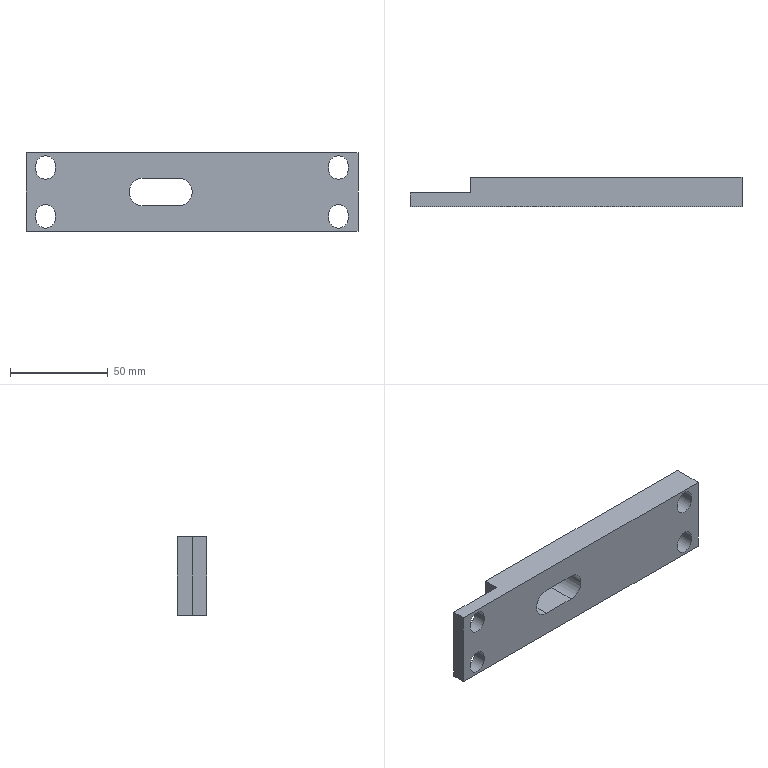Part | SolidWorks | features BaseBody 1 | 1 solid | 32 faces | box 170 x 15 x 40 mm | volume 81474 mm3 | plane 18 | cylinder 14 | commonest cylinder face diameters 10 x12 14.3 x2
STEP:
#1=CARTESIAN_POINT('',(-75.,0.,-6.5));
#2=VERTEX_POINT('',#1);
#3=CARTESIAN_POINT('',(-70.,0.,-11.5));
#4=VERTEX_POINT('',#3);
#5=CARTESIAN_POINT('',(-75.,0.,-11.5));
#6=DIRECTION('',(0.,1.,0.));
#7=DIRECTION('',(0.,0.,1.));
#8=AXIS2_PLACEMENT_3D('',#5,#6,#7);
#9=CIRCLE('',#8,5.);
#10=EDGE_CURVE('',#2,#4,#9,.T.);
#11=ORIENTED_EDGE('',*,*,#10,.F.);
#12=CARTESIAN_POINT('',(-75.,7.,-6.5));
#13=VERTEX_POINT('',#12);
#14=CARTESIAN_POINT('',(-75.,0.,-6.5));
#15=DIRECTION('',(0.,1.,0.));
#16=VECTOR('',#15,1000.);
#17=LINE('',#14,#16);
#18=EDGE_CURVE('',#2,#13,#17,.T.);
#19=ORIENTED_EDGE('',*,*,#18,.T.);
#20=CARTESIAN_POINT('',(-70.,7.,-11.5));
#21=VERTEX_POINT('',#20);
#22=CARTESIAN_POINT('',(-75.,7.,-11.5));
#23=DIRECTION('',(0.,-1.,0.));
#24=DIRECTION('',(0.,0.,1.));
#25=AXIS2_PLACEMENT_3D('',#22,#23,#24);
#26=CIRCLE('',#25,5.);
#27=EDGE_CURVE('',#21,#13,#26,.T.);
#28=ORIENTED_EDGE('',*,*,#27,.F.);
#29=CARTESIAN_POINT('',(-70.,0.,-11.5));
#30=DIRECTION('',(0.,-1.,0.));
#31=VECTOR('',#30,1000.);
#32=LINE('',#29,#31);
#33=EDGE_CURVE('',#21,#4,#32,.T.);
#34=ORIENTED_EDGE('',*,*,#33,.T.);
#35=EDGE_LOOP('',(#11,#19,#28,#34));
#36=FACE_OUTER_BOUND('',#35,.T.);
#37=CARTESIAN_POINT('',(-75.,0.,-11.5));
#38=DIRECTION('',(0.,1.,0.));
#39=DIRECTION('',(0.,0.,1.));
#40=AXIS2_PLACEMENT_3D('',#37,#38,#39);
#41=CYLINDRICAL_SURFACE('',#40,5.);
#42=ADVANCED_FACE('',(#36),#41,.F.);
#43=CARTESIAN_POINT('',(75.,0.,18.5));
#44=VERTEX_POINT('',#43);
#45=CARTESIAN_POINT('',(80.,0.,13.5));
#46=VERTEX_POINT('',#45);
#47=CARTESIAN_POINT('',(75.,0.,13.5));
#48=DIRECTION('',(0.,1.,0.));
#49=DIRECTION('',(0.,0.,1.));
#50=AXIS2_PLACEMENT_3D('',#47,#48,#49);
#51=CIRCLE('',#50,5.);
#52=EDGE_CURVE('',#44,#46,#51,.T.);
#53=ORIENTED_EDGE('',*,*,#52,.F.);
#54=CARTESIAN_POINT('',(75.,15.,18.5));
#55=VERTEX_POINT('',#54);
#56=CARTESIAN_POINT('',(75.,0.,18.5));
#57=DIRECTION('',(0.,1.,0.));
#58=VECTOR('',#57,1000.);
#59=LINE('',#56,#58);
#60=EDGE_CURVE('',#44,#55,#59,.T.);
#61=ORIENTED_EDGE('',*,*,#60,.T.);
#62=CARTESIAN_POINT('',(80.,15.,13.5));
#63=VERTEX_POINT('',#62);
#64=CARTESIAN_POINT('',(75.,15.,13.5));
#65=DIRECTION('',(0.,-1.,0.));
#66=DIRECTION('',(0.,0.,1.));
#67=AXIS2_PLACEMENT_3D('',#64,#65,#66);
#68=CIRCLE('',#67,5.);
#69=EDGE_CURVE('',#63,#55,#68,.T.);
#70=ORIENTED_EDGE('',*,*,#69,.F.);
#71=CARTESIAN_POINT('',(80.,0.,13.5));
#72=DIRECTION('',(0.,-1.,0.));
#73=VECTOR('',#72,1000.);
#74=LINE('',#71,#73);
#75=EDGE_CURVE('',#63,#46,#74,.T.);
#76=ORIENTED_EDGE('',*,*,#75,.T.);
#77=EDGE_LOOP('',(#53,#61,#70,#76));
#78=FACE_OUTER_BOUND('',#77,.T.);
#79=CARTESIAN_POINT('',(75.,0.,13.5));
#80=DIRECTION('',(0.,1.,0.));
#81=DIRECTION('',(0.,0.,1.));
#82=AXIS2_PLACEMENT_3D('',#79,#80,#81);
#83=CYLINDRICAL_SURFACE('',#82,5.);
#84=ADVANCED_FACE('',(#78),#83,.F.);
#85=CARTESIAN_POINT('',(-75.,0.,18.5));
#86=VERTEX_POINT('',#85);
#87=CARTESIAN_POINT('',(-70.,0.,13.5));
#88=VERTEX_POINT('',#87);
#89=CARTESIAN_POINT('',(-75.,0.,13.5));
#90=DIRECTION('',(0.,1.,0.));
#91=DIRECTION('',(0.,0.,1.));
#92=AXIS2_PLACEMENT_3D('',#89,#90,#91);
#93=CIRCLE('',#92,5.);
#94=EDGE_CURVE('',#86,#88,#93,.T.);
#95=ORIENTED_EDGE('',*,*,#94,.F.);
#96=CARTESIAN_POINT('',(-75.,7.,18.5));
#97=VERTEX_POINT('',#96);
#98=CARTESIAN_POINT('',(-75.,0.,18.5));
#99=DIRECTION('',(0.,1.,0.));
#100=VECTOR('',#99,1000.);
#101=LINE('',#98,#100);
#102=EDGE_CURVE('',#86,#97,#101,.T.);
#103=ORIENTED_EDGE('',*,*,#102,.T.);
#104=CARTESIAN_POINT('',(-70.,7.,13.5));
#105=VERTEX_POINT('',#104);
#106=CARTESIAN_POINT('',(-75.,7.,13.5));
#107=DIRECTION('',(0.,-1.,0.));
#108=DIRECTION('',(0.,0.,1.));
#109=AXIS2_PLACEMENT_3D('',#106,#107,#108);
#110=CIRCLE('',#109,5.);
#111=EDGE_CURVE('',#105,#97,#110,.T.);
#112=ORIENTED_EDGE('',*,*,#111,.F.);
#113=CARTESIAN_POINT('',(-70.,0.,13.5));
#114=DIRECTION('',(0.,-1.,0.));
#115=VECTOR('',#114,1000.);
#116=LINE('',#113,#115);
#117=EDGE_CURVE('',#105,#88,#116,.T.);
#118=ORIENTED_EDGE('',*,*,#117,.T.);
#119=EDGE_LOOP('',(#95,#103,#112,#118));
#120=FACE_OUTER_BOUND('',#119,.T.);
#121=CARTESIAN_POINT('',(-75.,0.,13.5));
#122=DIRECTION('',(0.,1.,0.));
#123=DIRECTION('',(0.,0.,1.));
#124=AXIS2_PLACEMENT_3D('',#121,#122,#123);
#125=CYLINDRICAL_SURFACE('',#124,5.);
#126=ADVANCED_FACE('',(#120),#125,.F.);
#127=CARTESIAN_POINT('',(75.,0.,-6.5));
#128=VERTEX_POINT('',#127);
#129=CARTESIAN_POINT('',(80.,0.,-11.5));
#130=VERTEX_POINT('',#129);
#131=CARTESIAN_POINT('',(75.,0.,-11.5));
#132=DIRECTION('',(0.,1.,0.));
#133=DIRECTION('',(0.,0.,1.));
#134=AXIS2_PLACEMENT_3D('',#131,#132,#133);
#135=CIRCLE('',#134,5.);
#136=EDGE_CURVE('',#128,#130,#135,.T.);
#137=ORIENTED_EDGE('',*,*,#136,.F.);
#138=CARTESIAN_POINT('',(75.,15.,-6.5));
#139=VERTEX_POINT('',#138);
#140=CARTESIAN_POINT('',(75.,0.,-6.5));
#141=DIRECTION('',(0.,1.,0.));
#142=VECTOR('',#141,1000.);
#143=LINE('',#140,#142);
#144=EDGE_CURVE('',#128,#139,#143,.T.);
#145=ORIENTED_EDGE('',*,*,#144,.T.);
#146=CARTESIAN_POINT('',(80.,15.,-11.5));
#147=VERTEX_POINT('',#146);
#148=CARTESIAN_POINT('',(75.,15.,-11.5));
#149=DIRECTION('',(0.,-1.,0.));
#150=DIRECTION('',(0.,0.,1.));
#151=AXIS2_PLACEMENT_3D('',#148,#149,#150);
#152=CIRCLE('',#151,5.);
#153=EDGE_CURVE('',#147,#139,#152,.T.);
#154=ORIENTED_EDGE('',*,*,#153,.F.);
#155=CARTESIAN_POINT('',(80.,0.,-11.5));
#156=DIRECTION('',(0.,-1.,0.));
#157=VECTOR('',#156,1000.);
#158=LINE('',#155,#157);
#159=EDGE_CURVE('',#147,#130,#158,.T.);
#160=ORIENTED_EDGE('',*,*,#159,.T.);
#161=EDGE_LOOP('',(#137,#145,#154,#160));
#162=FACE_OUTER_BOUND('',#161,.T.);
#163=CARTESIAN_POINT('',(75.,0.,-11.5));
#164=DIRECTION('',(0.,1.,0.));
#165=DIRECTION('',(0.,0.,1.));
#166=AXIS2_PLACEMENT_3D('',#163,#164,#165);
#167=CYLINDRICAL_SURFACE('',#166,5.);
#168=ADVANCED_FACE('',(#162),#167,.F.);
#169=CARTESIAN_POINT('',(-85.,0.,20.));
#170=VERTEX_POINT('',#169);
#171=CARTESIAN_POINT('',(-85.,0.,-20.));
#172=VERTEX_POINT('',#171);
#173=CARTESIAN_POINT('',(-85.,0.,0.));
#174=DIRECTION('',(0.,0.,-1.));
#175=VECTOR('',#174,1000.);
#176=LINE('',#173,#175);
#177=EDGE_CURVE('',#170,#172,#176,.T.);
#178=ORIENTED_EDGE('',*,*,#177,.T.);
#179=CARTESIAN_POINT('',(85.,0.,-20.));
#180=VERTEX_POINT('',#179);
#181=CARTESIAN_POINT('',(0.,0.,-20.));
#182=DIRECTION('',(1.,0.,0.));
#183=VECTOR('',#182,1000.);
#184=LINE('',#181,#183);
#185=EDGE_CURVE('',#172,#180,#184,.T.);
#186=ORIENTED_EDGE('',*,*,#185,.T.);
#187=CARTESIAN_POINT('',(85.,0.,20.));
#188=VERTEX_POINT('',#187);
#189=CARTESIAN_POINT('',(85.,0.,0.));
#190=DIRECTION('',(0.,0.,1.));
#191=VECTOR('',#190,1000.);
#192=LINE('',#189,#191);
#193=EDGE_CURVE('',#180,#188,#192,.T.);
#194=ORIENTED_EDGE('',*,*,#193,.T.);
#195=CARTESIAN_POINT('',(0.,0.,20.));
#196=DIRECTION('',(-1.,0.,0.));
#197=VECTOR('',#196,1000.);
#198=LINE('',#195,#197);
#199=EDGE_CURVE('',#188,#170,#198,.T.);
#200=ORIENTED_EDGE('',*,*,#199,.T.);
#201=EDGE_LOOP('',(#178,#186,#194,#200));
#202=FACE_OUTER_BOUND('',#201,.T.);
#203=CARTESIAN_POINT('',(-25.,0.,-7.15));
#204=VERTEX_POINT('',#203);
#205=CARTESIAN_POINT('',(-25.,0.,7.15));
#206=VERTEX_POINT('',#205);
#207=CARTESIAN_POINT('',(-25.,0.,0.));
#208=DIRECTION('',(0.,1.,0.));
#209=DIRECTION('',(0.,0.,1.));
#210=AXIS2_PLACEMENT_3D('',#207,#208,#209);
#211=CIRCLE('',#210,7.15);
#212=EDGE_CURVE('',#204,#206,#211,.T.);
#213=ORIENTED_EDGE('',*,*,#212,.T.);
#214=CARTESIAN_POINT('',(-7.,0.,7.15));
#215=VERTEX_POINT('',#214);
#216=CARTESIAN_POINT('',(0.,0.,7.15));
#217=DIRECTION('',(1.,0.,0.));
#218=VECTOR('',#217,1000.);
#219=LINE('',#216,#218);
#220=EDGE_CURVE('',#206,#215,#219,.T.);
#221=ORIENTED_EDGE('',*,*,#220,.T.);
#222=CARTESIAN_POINT('',(-7.,0.,-7.15));
#223=VERTEX_POINT('',#222);
#224=CARTESIAN_POINT('',(-7.,0.,0.));
#225=DIRECTION('',(0.,1.,0.));
#226=DIRECTION('',(0.,0.,1.));
#227=AXIS2_PLACEMENT_3D('',#224,#225,#226);
#228=CIRCLE('',#227,7.15);
#229=EDGE_CURVE('',#215,#223,#228,.T.);
#230=ORIENTED_EDGE('',*,*,#229,.T.);
#231=CARTESIAN_POINT('',(0.,0.,-7.15));
#232=DIRECTION('',(-1.,0.,0.));
#233=VECTOR('',#232,1000.);
#234=LINE('',#231,#233);
#235=EDGE_CURVE('',#223,#204,#234,.T.);
#236=ORIENTED_EDGE('',*,*,#235,.T.);
#237=EDGE_LOOP('',(#213,#221,#230,#236));
#238=FACE_BOUND('',#237,.T.);
#239=CARTESIAN_POINT('',(-80.,0.,-11.5));
#240=VERTEX_POINT('',#239);
#241=CARTESIAN_POINT('',(-75.,0.,-11.5));
#242=DIRECTION('',(0.,1.,0.));
#243=DIRECTION('',(0.,0.,1.));
#244=AXIS2_PLACEMENT_3D('',#241,#242,#243);
#245=CIRCLE('',#244,5.);
#246=EDGE_CURVE('',#240,#2,#245,.T.);
#247=ORIENTED_EDGE('',*,*,#246,.T.);
#248=ORIENTED_EDGE('',*,*,#10,.T.);
#249=CARTESIAN_POINT('',(-70.,0.,-13.5));
#250=VERTEX_POINT('',#249);
#251=CARTESIAN_POINT('',(-70.,0.,0.));
#252=DIRECTION('',(0.,0.,-1.));
#253=VECTOR('',#252,1000.);
#254=LINE('',#251,#253);
#255=EDGE_CURVE('',#4,#250,#254,.T.);
#256=ORIENTED_EDGE('',*,*,#255,.T.);
#257=CARTESIAN_POINT('',(-80.,0.,-13.5));
#258=VERTEX_POINT('',#257);
#259=CARTESIAN_POINT('',(-75.,0.,-13.5));
#260=DIRECTION('',(0.,1.,0.));
#261=DIRECTION('',(0.,0.,1.));
#262=AXIS2_PLACEMENT_3D('',#259,#260,#261);
#263=CIRCLE('',#262,5.);
#264=EDGE_CURVE('',#250,#258,#263,.T.);
#265=ORIENTED_EDGE('',*,*,#264,.T.);
#266=CARTESIAN_POINT('',(-80.,0.,0.));
#267=DIRECTION('',(0.,0.,1.));
#268=VECTOR('',#267,1000.);
#269=LINE('',#266,#268);
#270=EDGE_CURVE('',#258,#240,#269,.T.);
#271=ORIENTED_EDGE('',*,*,#270,.T.);
#272=EDGE_LOOP('',(#247,#248,#256,#265,#271));
#273=FACE_BOUND('',#272,.T.);
#274=CARTESIAN_POINT('',(80.,0.,11.5));
#275=VERTEX_POINT('',#274);
#276=CARTESIAN_POINT('',(70.,0.,11.5));
#277=VERTEX_POINT('',#276);
#278=CARTESIAN_POINT('',(75.,0.,11.5));
#279=DIRECTION('',(0.,1.,0.));
#280=DIRECTION('',(0.,0.,1.));
#281=AXIS2_PLACEMENT_3D('',#278,#279,#280);
#282=CIRCLE('',#281,5.);
#283=EDGE_CURVE('',#275,#277,#282,.T.);
#284=ORIENTED_EDGE('',*,*,#283,.T.);
#285=CARTESIAN_POINT('',(70.,0.,13.5));
#286=VERTEX_POINT('',#285);
#287=CARTESIAN_POINT('',(70.,0.,0.));
#288=DIRECTION('',(0.,0.,1.));
#289=VECTOR('',#288,1000.);
#290=LINE('',#287,#289);
#291=EDGE_CURVE('',#277,#286,#290,.T.);
#292=ORIENTED_EDGE('',*,*,#291,.T.);
#293=CARTESIAN_POINT('',(75.,0.,13.5));
#294=DIRECTION('',(0.,1.,0.));
#295=DIRECTION('',(0.,0.,1.));
#296=AXIS2_PLACEMENT_3D('',#293,#294,#295);
#297=CIRCLE('',#296,5.);
#298=EDGE_CURVE('',#286,#44,#297,.T.);
#299=ORIENTED_EDGE('',*,*,#298,.T.);
#300=ORIENTED_EDGE('',*,*,#52,.T.);
#301=CARTESIAN_POINT('',(80.,0.,0.));
#302=DIRECTION('',(0.,0.,-1.));
#303=VECTOR('',#302,1000.);
#304=LINE('',#301,#303);
#305=EDGE_CURVE('',#46,#275,#304,.T.);
#306=ORIENTED_EDGE('',*,*,#305,.T.);
#307=EDGE_LOOP('',(#284,#292,#299,#300,#306));
#308=FACE_BOUND('',#307,.T.);
#309=CARTESIAN_POINT('',(-70.,0.,11.5));
#310=VERTEX_POINT('',#309);
#311=CARTESIAN_POINT('',(-80.,0.,11.5));
#312=VERTEX_POINT('',#311);
#313=CARTESIAN_POINT('',(-75.,0.,11.5));
#314=DIRECTION('',(0.,1.,0.));
#315=DIRECTION('',(0.,0.,1.));
#316=AXIS2_PLACEMENT_3D('',#313,#314,#315);
#317=CIRCLE('',#316,5.);
#318=EDGE_CURVE('',#310,#312,#317,.T.);
#319=ORIENTED_EDGE('',*,*,#318,.T.);
#320=CARTESIAN_POINT('',(-80.,0.,13.5));
#321=VERTEX_POINT('',#320);
#322=CARTESIAN_POINT('',(-80.,0.,0.));
#323=DIRECTION('',(0.,0.,1.));
#324=VECTOR('',#323,1000.);
#325=LINE('',#322,#324);
#326=EDGE_CURVE('',#312,#321,#325,.T.);
#327=ORIENTED_EDGE('',*,*,#326,.T.);
#328=CARTESIAN_POINT('',(-75.,0.,13.5));
#329=DIRECTION('',(0.,1.,0.));
#330=DIRECTION('',(0.,0.,1.));
#331=AXIS2_PLACEMENT_3D('',#328,#329,#330);
#332=CIRCLE('',#331,5.);
#333=EDGE_CURVE('',#321,#86,#332,.T.);
#334=ORIENTED_EDGE('',*,*,#333,.T.);
#335=ORIENTED_EDGE('',*,*,#94,.T.);
#336=CARTESIAN_POINT('',(-70.,0.,0.));
#337=DIRECTION('',(0.,0.,-1.));
#338=VECTOR('',#337,1000.);
#339=LINE('',#336,#338);
#340=EDGE_CURVE('',#88,#310,#339,.T.);
#341=ORIENTED_EDGE('',*,*,#340,.T.);
#342=EDGE_LOOP('',(#319,#327,#334,#335,#341));
#343=FACE_BOUND('',#342,.T.);
#344=CARTESIAN_POINT('',(70.,0.,-11.5));
#345=VERTEX_POINT('',#344);
#346=CARTESIAN_POINT('',(75.,0.,-11.5));
#347=DIRECTION('',(0.,1.,0.));
#348=DIRECTION('',(0.,0.,1.));
#349=AXIS2_PLACEMENT_3D('',#346,#347,#348);
#350=CIRCLE('',#349,5.);
#351=EDGE_CURVE('',#345,#128,#350,.T.);
#352=ORIENTED_EDGE('',*,*,#351,.T.);
#353=ORIENTED_EDGE('',*,*,#136,.T.);
#354=CARTESIAN_POINT('',(80.,0.,-13.5));
#355=VERTEX_POINT('',#354);
#356=CARTESIAN_POINT('',(80.,0.,0.));
#357=DIRECTION('',(0.,0.,-1.));
#358=VECTOR('',#357,1000.);
#359=LINE('',#356,#358);
#360=EDGE_CURVE('',#130,#355,#359,.T.);
#361=ORIENTED_EDGE('',*,*,#360,.T.);
#362=CARTESIAN_POINT('',(70.,0.,-13.5));
#363=VERTEX_POINT('',#362);
#364=CARTESIAN_POINT('',(75.,0.,-13.5));
#365=DIRECTION('',(0.,1.,0.));
#366=DIRECTION('',(0.,0.,1.));
#367=AXIS2_PLACEMENT_3D('',#364,#365,#366);
#368=CIRCLE('',#367,5.);
#369=EDGE_CURVE('',#355,#363,#368,.T.);
#370=ORIENTED_EDGE('',*,*,#369,.T.);
#371=CARTESIAN_POINT('',(70.,0.,0.));
#372=DIRECTION('',(0.,0.,1.));
#373=VECTOR('',#372,1000.);
#374=LINE('',#371,#373);
#375=EDGE_CURVE('',#363,#345,#374,.T.);
#376=ORIENTED_EDGE('',*,*,#375,.T.);
#377=EDGE_LOOP('',(#352,#353,#361,#370,#376));
#378=FACE_BOUND('',#377,.T.);
#379=CARTESIAN_POINT('',(0.,0.,0.));
#380=DIRECTION('',(0.,-1.,0.));
#381=DIRECTION('',(0.,0.,-1.));
#382=AXIS2_PLACEMENT_3D('',#379,#380,#381);
#383=PLANE('',#382);
#384=ADVANCED_FACE('',(#202,#238,#273,#308,#343,#378),#383,.T.);
#385=CARTESIAN_POINT('',(-54.,15.,-20.));
#386=VERTEX_POINT('',#385);
#387=CARTESIAN_POINT('',(-54.,7.,-20.));
#388=VERTEX_POINT('',#387);
#389=CARTESIAN_POINT('',(-54.,15.,-20.));
#390=DIRECTION('',(0.,-1.,0.));
#391=VECTOR('',#390,1000.);
#392=LINE('',#389,#391);
#393=EDGE_CURVE('',#386,#388,#392,.T.);
#394=ORIENTED_EDGE('',*,*,#393,.F.);
#395=CARTESIAN_POINT('',(85.,15.,-20.));
#396=VERTEX_POINT('',#395);
#397=CARTESIAN_POINT('',(-85.,15.,-20.));
#398=DIRECTION('',(-1.,0.,0.));
#399=VECTOR('',#398,1000.);
#400=LINE('',#397,#399);
#401=EDGE_CURVE('',#396,#386,#400,.T.);
#402=ORIENTED_EDGE('',*,*,#401,.F.);
#403=CARTESIAN_POINT('',(85.,15.,-20.));
#404=DIRECTION('',(0.,1.,0.));
#405=VECTOR('',#404,1000.);
#406=LINE('',#403,#405);
#407=EDGE_CURVE('',#180,#396,#406,.T.);
#408=ORIENTED_EDGE('',*,*,#407,.F.);
#409=ORIENTED_EDGE('',*,*,#185,.F.);
#410=CARTESIAN_POINT('',(-85.,7.,-20.));
#411=VERTEX_POINT('',#410);
#412=CARTESIAN_POINT('',(-85.,15.,-20.));
#413=DIRECTION('',(0.,-1.,0.));
#414=VECTOR('',#413,1000.);
#415=LINE('',#412,#414);
#416=EDGE_CURVE('',#411,#172,#415,.T.);
#417=ORIENTED_EDGE('',*,*,#416,.F.);
#418=CARTESIAN_POINT('',(-85.,7.,-20.));
#419=DIRECTION('',(-1.,0.,0.));
#420=VECTOR('',#419,1000.);
#421=LINE('',#418,#420);
#422=EDGE_CURVE('',#388,#411,#421,.T.);
#423=ORIENTED_EDGE('',*,*,#422,.F.);
#424=EDGE_LOOP('',(#394,#402,#408,#409,#417,#423));
#425=FACE_OUTER_BOUND('',#424,.T.);
#426=CARTESIAN_POINT('',(-85.,15.,-20.));
#427=DIRECTION('',(0.,0.,1.));
#428=DIRECTION('',(1.,0.,0.));
#429=AXIS2_PLACEMENT_3D('',#426,#427,#428);
#430=PLANE('',#429);
#431=ADVANCED_FACE('',(#425),#430,.F.);
#432=CARTESIAN_POINT('',(-85.,7.,20.));
#433=VERTEX_POINT('',#432);
#434=CARTESIAN_POINT('',(-85.,7.,20.));
#435=DIRECTION('',(0.,0.,1.));
#436=VECTOR('',#435,1000.);
#437=LINE('',#434,#436);
#438=EDGE_CURVE('',#411,#433,#437,.T.);
#439=ORIENTED_EDGE('',*,*,#438,.F.);
#440=ORIENTED_EDGE('',*,*,#416,.T.);
#441=ORIENTED_EDGE('',*,*,#177,.F.);
#442=CARTESIAN_POINT('',(-85.,15.,20.));
#443=DIRECTION('',(0.,-1.,0.));
#444=VECTOR('',#443,1000.);
#445=LINE('',#442,#444);
#446=EDGE_CURVE('',#433,#170,#445,.T.);
#447=ORIENTED_EDGE('',*,*,#446,.F.);
#448=EDGE_LOOP('',(#439,#440,#441,#447));
#449=FACE_OUTER_BOUND('',#448,.T.);
#450=CARTESIAN_POINT('',(-85.,15.,20.));
#451=DIRECTION('',(1.,0.,0.));
#452=DIRECTION('',(0.,0.,-1.));
#453=AXIS2_PLACEMENT_3D('',#450,#451,#452);
#454=PLANE('',#453);
#455=ADVANCED_FACE('',(#449),#454,.F.);
#456=CARTESIAN_POINT('',(-54.,7.,20.));
#457=VERTEX_POINT('',#456);
#458=CARTESIAN_POINT('',(-54.,15.,20.));
#459=VERTEX_POINT('',#458);
#460=CARTESIAN_POINT('',(-54.,15.,20.));
#461=DIRECTION('',(0.,1.,0.));
#462=VECTOR('',#461,1000.);
#463=LINE('',#460,#462);
#464=EDGE_CURVE('',#457,#459,#463,.T.);
#465=ORIENTED_EDGE('',*,*,#464,.F.);
#466=CARTESIAN_POINT('',(-85.,7.,20.));
#467=DIRECTION('',(1.,0.,0.));
#468=VECTOR('',#467,1000.);
#469=LINE('',#466,#468);
#470=EDGE_CURVE('',#433,#457,#469,.T.);
#471=ORIENTED_EDGE('',*,*,#470,.F.);
#472=ORIENTED_EDGE('',*,*,#446,.T.);
#473=ORIENTED_EDGE('',*,*,#199,.F.);
#474=CARTESIAN_POINT('',(85.,15.,20.));
#475=VERTEX_POINT('',#474);
#476=CARTESIAN_POINT('',(85.,15.,20.));
#477=DIRECTION('',(0.,-1.,0.));
#478=VECTOR('',#477,1000.);
#479=LINE('',#476,#478);
#480=EDGE_CURVE('',#475,#188,#479,.T.);
#481=ORIENTED_EDGE('',*,*,#480,.F.);
#482=CARTESIAN_POINT('',(-85.,15.,20.));
#483=DIRECTION('',(1.,0.,0.));
#484=VECTOR('',#483,1000.);
#485=LINE('',#482,#484);
#486=EDGE_CURVE('',#459,#475,#485,.T.);
#487=ORIENTED_EDGE('',*,*,#486,.F.);
#488=EDGE_LOOP('',(#465,#471,#472,#473,#481,#487));
#489=FACE_OUTER_BOUND('',#488,.T.);
#490=CARTESIAN_POINT('',(-85.,15.,20.));
#491=DIRECTION('',(0.,0.,-1.));
#492=DIRECTION('',(-1.,0.,0.));
#493=AXIS2_PLACEMENT_3D('',#490,#491,#492);
#494=PLANE('',#493);
#495=ADVANCED_FACE('',(#489),#494,.F.);
#496=ORIENTED_EDGE('',*,*,#407,.T.);
#497=CARTESIAN_POINT('',(85.,15.,20.));
#498=DIRECTION('',(0.,0.,-1.));
#499=VECTOR('',#498,1000.);
#500=LINE('',#497,#499);
#501=EDGE_CURVE('',#475,#396,#500,.T.);
#502=ORIENTED_EDGE('',*,*,#501,.F.);
#503=ORIENTED_EDGE('',*,*,#480,.T.);
#504=ORIENTED_EDGE('',*,*,#193,.F.);
#505=EDGE_LOOP('',(#496,#502,#503,#504));
#506=FACE_OUTER_BOUND('',#505,.T.);
#507=CARTESIAN_POINT('',(85.,15.,20.));
#508=DIRECTION('',(-1.,0.,0.));
#509=DIRECTION('',(0.,0.,1.));
#510=AXIS2_PLACEMENT_3D('',#507,#508,#509);
#511=PLANE('',#510);
#512=ADVANCED_FACE('',(#506),#511,.F.);
#513=CARTESIAN_POINT('',(-7.,15.,7.15));
#514=VERTEX_POINT('',#513);
#515=CARTESIAN_POINT('',(-7.,0.,7.15));
#516=DIRECTION('',(0.,1.,0.));
#517=VECTOR('',#516,1000.);
#518=LINE('',#515,#517);
#519=EDGE_CURVE('',#215,#514,#518,.T.);
#520=ORIENTED_EDGE('',*,*,#519,.F.);
#521=ORIENTED_EDGE('',*,*,#220,.F.);
#522=CARTESIAN_POINT('',(-25.,15.,7.15));
#523=VERTEX_POINT('',#522);
#524=CARTESIAN_POINT('',(-25.,0.,7.15));
#525=DIRECTION('',(0.,-1.,0.));
#526=VECTOR('',#525,1000.);
#527=LINE('',#524,#526);
#528=EDGE_CURVE('',#523,#206,#527,.T.);
#529=ORIENTED_EDGE('',*,*,#528,.F.);
#530=CARTESIAN_POINT('',(-7.,15.,7.15));
#531=DIRECTION('',(-1.,0.,0.));
#532=VECTOR('',#531,1000.);
#533=LINE('',#530,#532);
#534=EDGE_CURVE('',#514,#523,#533,.T.);
#535=ORIENTED_EDGE('',*,*,#534,.F.);
#536=EDGE_LOOP('',(#520,#521,#529,#535));
#537=FACE_OUTER_BOUND('',#536,.T.);
#538=CARTESIAN_POINT('',(-7.,0.,7.15));
#539=DIRECTION('',(0.,0.,1.));
#540=DIRECTION('',(1.,0.,0.));
#541=AXIS2_PLACEMENT_3D('',#538,#539,#540);
#542=PLANE('',#541);
#543=ADVANCED_FACE('',(#537),#542,.F.);
#544=ORIENTED_EDGE('',*,*,#528,.T.);
#545=ORIENTED_EDGE('',*,*,#212,.F.);
#546=CARTESIAN_POINT('',(-25.,15.,-7.15));
#547=VERTEX_POINT('',#546);
#548=CARTESIAN_POINT('',(-25.,0.,-7.15));
#549=DIRECTION('',(0.,-1.,0.));
#550=VECTOR('',#549,1000.);
#551=LINE('',#548,#550);
#552=EDGE_CURVE('',#547,#204,#551,.T.);
#553=ORIENTED_EDGE('',*,*,#552,.F.);
#554=CARTESIAN_POINT('',(-25.,15.,0.));
#555=DIRECTION('',(0.,-1.,0.));
#556=DIRECTION('',(0.,0.,1.));
#557=AXIS2_PLACEMENT_3D('',#554,#555,#556);
#558=CIRCLE('',#557,7.15);
#559=EDGE_CURVE('',#523,#547,#558,.T.);
#560=ORIENTED_EDGE('',*,*,#559,.F.);
#561=EDGE_LOOP('',(#544,#545,#553,#560));
#562=FACE_OUTER_BOUND('',#561,.T.);
#563=CARTESIAN_POINT('',(-25.,0.,0.));
#564=DIRECTION('',(0.,1.,0.));
#565=DIRECTION('',(0.,0.,1.));
#566=AXIS2_PLACEMENT_3D('',#563,#564,#565);
#567=CYLINDRICAL_SURFACE('',#566,7.15);
#568=ADVANCED_FACE('',(#562),#567,.F.);
#569=ORIENTED_EDGE('',*,*,#552,.T.);
#570=ORIENTED_EDGE('',*,*,#235,.F.);
#571=CARTESIAN_POINT('',(-7.,15.,-7.15));
#572=VERTEX_POINT('',#571);
#573=CARTESIAN_POINT('',(-7.,0.,-7.15));
#574=DIRECTION('',(0.,-1.,0.));
#575=VECTOR('',#574,1000.);
#576=LINE('',#573,#575);
#577=EDGE_CURVE('',#572,#223,#576,.T.);
#578=ORIENTED_EDGE('',*,*,#577,.F.);
#579=CARTESIAN_POINT('',(-7.,15.,-7.15));
#580=DIRECTION('',(1.,0.,0.));
#581=VECTOR('',#580,1000.);
#582=LINE('',#579,#581);
#583=EDGE_CURVE('',#547,#572,#582,.T.);
#584=ORIENTED_EDGE('',*,*,#583,.F.);
#585=EDGE_LOOP('',(#569,#570,#578,#584));
#586=FACE_OUTER_BOUND('',#585,.T.);
#587=CARTESIAN_POINT('',(-7.,0.,-7.15));
#588=DIRECTION('',(0.,0.,-1.));
#589=DIRECTION('',(-1.,0.,0.));
#590=AXIS2_PLACEMENT_3D('',#587,#588,#589);
#591=PLANE('',#590);
#592=ADVANCED_FACE('',(#586),#591,.F.);
#593=ORIENTED_EDGE('',*,*,#577,.T.);
#594=ORIENTED_EDGE('',*,*,#229,.F.);
#595=ORIENTED_EDGE('',*,*,#519,.T.);
#596=CARTESIAN_POINT('',(-7.,15.,0.));
#597=DIRECTION('',(0.,-1.,0.));
#598=DIRECTION('',(0.,0.,1.));
#599=AXIS2_PLACEMENT_3D('',#596,#597,#598);
#600=CIRCLE('',#599,7.15);
#601=EDGE_CURVE('',#572,#514,#600,.T.);
#602=ORIENTED_EDGE('',*,*,#601,.F.);
#603=EDGE_LOOP('',(#593,#594,#595,#602));
#604=FACE_OUTER_BOUND('',#603,.T.);
#605=CARTESIAN_POINT('',(-7.,0.,0.));
#606=DIRECTION('',(0.,1.,0.));
#607=DIRECTION('',(0.,0.,1.));
#608=AXIS2_PLACEMENT_3D('',#605,#606,#607);
#609=CYLINDRICAL_SURFACE('',#608,7.15);
#610=ADVANCED_FACE('',(#604),#609,.F.);
#611=CARTESIAN_POINT('',(-70.,7.,-13.5));
#612=VERTEX_POINT('',#611);
#613=CARTESIAN_POINT('',(-70.,7.,-13.5));
#614=DIRECTION('',(0.,0.,1.));
#615=VECTOR('',#614,1000.);
#616=LINE('',#613,#615);
#617=EDGE_CURVE('',#612,#21,#616,.T.);
#618=ORIENTED_EDGE('',*,*,#617,.F.);
#619=CARTESIAN_POINT('',(-70.,0.,-13.5));
#620=DIRECTION('',(0.,1.,0.));
#621=VECTOR('',#620,1000.);
#622=LINE('',#619,#621);
#623=EDGE_CURVE('',#250,#612,#622,.T.);
#624=ORIENTED_EDGE('',*,*,#623,.F.);
#625=ORIENTED_EDGE('',*,*,#255,.F.);
#626=ORIENTED_EDGE('',*,*,#33,.F.);
#627=EDGE_LOOP('',(#618,#624,#625,#626));
#628=FACE_OUTER_BOUND('',#627,.T.);
#629=CARTESIAN_POINT('',(-70.,0.,-13.5));
#630=DIRECTION('',(1.,0.,0.));
#631=DIRECTION('',(0.,0.,-1.));
#632=AXIS2_PLACEMENT_3D('',#629,#630,#631);
#633=PLANE('',#632);
#634=ADVANCED_FACE('',(#628),#633,.F.);
#635=ORIENTED_EDGE('',*,*,#18,.F.);
#636=ORIENTED_EDGE('',*,*,#246,.F.);
#637=CARTESIAN_POINT('',(-80.,7.,-11.5));
#638=VERTEX_POINT('',#637);
#639=CARTESIAN_POINT('',(-80.,0.,-11.5));
#640=DIRECTION('',(0.,-1.,0.));
#641=VECTOR('',#640,1000.);
#642=LINE('',#639,#641);
#643=EDGE_CURVE('',#638,#240,#642,.T.);
#644=ORIENTED_EDGE('',*,*,#643,.F.);
#645=CARTESIAN_POINT('',(-75.,7.,-11.5));
#646=DIRECTION('',(0.,-1.,0.));
#647=DIRECTION('',(0.,0.,1.));
#648=AXIS2_PLACEMENT_3D('',#645,#646,#647);
#649=CIRCLE('',#648,5.);
#650=EDGE_CURVE('',#13,#638,#649,.T.);
#651=ORIENTED_EDGE('',*,*,#650,.F.);
#652=EDGE_LOOP('',(#635,#636,#644,#651));
#653=FACE_OUTER_BOUND('',#652,.T.);
#654=CARTESIAN_POINT('',(-75.,0.,-11.5));
#655=DIRECTION('',(0.,1.,0.));
#656=DIRECTION('',(0.,0.,1.));
#657=AXIS2_PLACEMENT_3D('',#654,#655,#656);
#658=CYLINDRICAL_SURFACE('',#657,5.);
#659=ADVANCED_FACE('',(#653),#658,.F.);
#660=CARTESIAN_POINT('',(-80.,7.,-13.5));
#661=VERTEX_POINT('',#660);
#662=CARTESIAN_POINT('',(-80.,7.,-13.5));
#663=DIRECTION('',(0.,0.,-1.));
#664=VECTOR('',#663,1000.);
#665=LINE('',#662,#664);
#666=EDGE_CURVE('',#638,#661,#665,.T.);
#667=ORIENTED_EDGE('',*,*,#666,.F.);
#668=ORIENTED_EDGE('',*,*,#643,.T.);
#669=ORIENTED_EDGE('',*,*,#270,.F.);
#670=CARTESIAN_POINT('',(-80.,0.,-13.5));
#671=DIRECTION('',(0.,-1.,0.));
#672=VECTOR('',#671,1000.);
#673=LINE('',#670,#672);
#674=EDGE_CURVE('',#661,#258,#673,.T.);
#675=ORIENTED_EDGE('',*,*,#674,.F.);
#676=EDGE_LOOP('',(#667,#668,#669,#675));
#677=FACE_OUTER_BOUND('',#676,.T.);
#678=CARTESIAN_POINT('',(-80.,0.,-13.5));
#679=DIRECTION('',(-1.,0.,0.));
#680=DIRECTION('',(0.,0.,1.));
#681=AXIS2_PLACEMENT_3D('',#678,#679,#680);
#682=PLANE('',#681);
#683=ADVANCED_FACE('',(#677),#682,.F.);
#684=CARTESIAN_POINT('',(-75.,7.,-13.5));
#685=DIRECTION('',(0.,-1.,0.));
#686=DIRECTION('',(0.,0.,1.));
#687=AXIS2_PLACEMENT_3D('',#684,#685,#686);
#688=CIRCLE('',#687,5.);
#689=EDGE_CURVE('',#661,#612,#688,.T.);
#690=ORIENTED_EDGE('',*,*,#689,.F.);
#691=ORIENTED_EDGE('',*,*,#674,.T.);
#692=ORIENTED_EDGE('',*,*,#264,.F.);
#693=ORIENTED_EDGE('',*,*,#623,.T.);
#694=EDGE_LOOP('',(#690,#691,#692,#693));
#695=FACE_OUTER_BOUND('',#694,.T.);
#696=CARTESIAN_POINT('',(-75.,0.,-13.5));
#697=DIRECTION('',(0.,1.,0.));
#698=DIRECTION('',(0.,0.,1.));
#699=AXIS2_PLACEMENT_3D('',#696,#697,#698);
#700=CYLINDRICAL_SURFACE('',#699,5.);
#701=ADVANCED_FACE('',(#695),#700,.F.);
#702=CARTESIAN_POINT('',(70.,15.,13.5));
#703=VERTEX_POINT('',#702);
#704=CARTESIAN_POINT('',(70.,0.,13.5));
#705=DIRECTION('',(0.,1.,0.));
#706=VECTOR('',#705,1000.);
#707=LINE('',#704,#706);
#708=EDGE_CURVE('',#286,#703,#707,.T.);
#709=ORIENTED_EDGE('',*,*,#708,.F.);
#710=ORIENTED_EDGE('',*,*,#291,.F.);
#711=CARTESIAN_POINT('',(70.,15.,11.5));
#712=VERTEX_POINT('',#711);
#713=CARTESIAN_POINT('',(70.,0.,11.5));
#714=DIRECTION('',(0.,-1.,0.));
#715=VECTOR('',#714,1000.);
#716=LINE('',#713,#715);
#717=EDGE_CURVE('',#712,#277,#716,.T.);
#718=ORIENTED_EDGE('',*,*,#717,.F.);
#719=CARTESIAN_POINT('',(70.,15.,13.5));
#720=DIRECTION('',(0.,0.,-1.));
#721=VECTOR('',#720,1000.);
#722=LINE('',#719,#721);
#723=EDGE_CURVE('',#703,#712,#722,.T.);
#724=ORIENTED_EDGE('',*,*,#723,.F.);
#725=EDGE_LOOP('',(#709,#710,#718,#724));
#726=FACE_OUTER_BOUND('',#725,.T.);
#727=CARTESIAN_POINT('',(70.,0.,13.5));
#728=DIRECTION('',(-1.,0.,0.));
#729=DIRECTION('',(0.,0.,1.));
#730=AXIS2_PLACEMENT_3D('',#727,#728,#729);
#731=PLANE('',#730);
#732=ADVANCED_FACE('',(#726),#731,.F.);
#733=ORIENTED_EDGE('',*,*,#717,.T.);
#734=ORIENTED_EDGE('',*,*,#283,.F.);
#735=CARTESIAN_POINT('',(80.,15.,11.5));
#736=VERTEX_POINT('',#735);
#737=CARTESIAN_POINT('',(80.,0.,11.5));
#738=DIRECTION('',(0.,-1.,0.));
#739=VECTOR('',#738,1000.);
#740=LINE('',#737,#739);
#741=EDGE_CURVE('',#736,#275,#740,.T.);
#742=ORIENTED_EDGE('',*,*,#741,.F.);
#743=CARTESIAN_POINT('',(75.,15.,11.5));
#744=DIRECTION('',(0.,-1.,0.));
#745=DIRECTION('',(0.,0.,1.));
#746=AXIS2_PLACEMENT_3D('',#743,#744,#745);
#747=CIRCLE('',#746,5.);
#748=EDGE_CURVE('',#712,#736,#747,.T.);
#749=ORIENTED_EDGE('',*,*,#748,.F.);
#750=EDGE_LOOP('',(#733,#734,#742,#749));
#751=FACE_OUTER_BOUND('',#750,.T.);
#752=CARTESIAN_POINT('',(75.,0.,11.5));
#753=DIRECTION('',(0.,1.,0.));
#754=DIRECTION('',(0.,0.,1.));
#755=AXIS2_PLACEMENT_3D('',#752,#753,#754);
#756=CYLINDRICAL_SURFACE('',#755,5.);
#757=ADVANCED_FACE('',(#751),#756,.F.);
#758=ORIENTED_EDGE('',*,*,#741,.T.);
#759=ORIENTED_EDGE('',*,*,#305,.F.);
#760=ORIENTED_EDGE('',*,*,#75,.F.);
#761=CARTESIAN_POINT('',(80.,15.,13.5));
#762=DIRECTION('',(0.,0.,1.));
#763=VECTOR('',#762,1000.);
#764=LINE('',#761,#763);
#765=EDGE_CURVE('',#736,#63,#764,.T.);
#766=ORIENTED_EDGE('',*,*,#765,.F.);
#767=EDGE_LOOP('',(#758,#759,#760,#766));
#768=FACE_OUTER_BOUND('',#767,.T.);
#769=CARTESIAN_POINT('',(80.,0.,13.5));
#770=DIRECTION('',(1.,0.,0.));
#771=DIRECTION('',(0.,0.,-1.));
#772=AXIS2_PLACEMENT_3D('',#769,#770,#771);
#773=PLANE('',#772);
#774=ADVANCED_FACE('',(#768),#773,.F.);
#775=ORIENTED_EDGE('',*,*,#60,.F.);
#776=ORIENTED_EDGE('',*,*,#298,.F.);
#777=ORIENTED_EDGE('',*,*,#708,.T.);
#778=CARTESIAN_POINT('',(75.,15.,13.5));
#779=DIRECTION('',(0.,-1.,0.));
#780=DIRECTION('',(0.,0.,1.));
#781=AXIS2_PLACEMENT_3D('',#778,#779,#780);
#782=CIRCLE('',#781,5.);
#783=EDGE_CURVE('',#55,#703,#782,.T.);
#784=ORIENTED_EDGE('',*,*,#783,.F.);
#785=EDGE_LOOP('',(#775,#776,#777,#784));
#786=FACE_OUTER_BOUND('',#785,.T.);
#787=CARTESIAN_POINT('',(75.,0.,13.5));
#788=DIRECTION('',(0.,1.,0.));
#789=DIRECTION('',(0.,0.,1.));
#790=AXIS2_PLACEMENT_3D('',#787,#788,#789);
#791=CYLINDRICAL_SURFACE('',#790,5.);
#792=ADVANCED_FACE('',(#786),#791,.F.);
#793=CARTESIAN_POINT('',(-80.,7.,13.5));
#794=VERTEX_POINT('',#793);
#795=CARTESIAN_POINT('',(-80.,7.,11.5));
#796=VERTEX_POINT('',#795);
#797=CARTESIAN_POINT('',(-80.,7.,13.5));
#798=DIRECTION('',(0.,0.,-1.));
#799=VECTOR('',#798,1000.);
#800=LINE('',#797,#799);
#801=EDGE_CURVE('',#794,#796,#800,.T.);
#802=ORIENTED_EDGE('',*,*,#801,.F.);
#803=CARTESIAN_POINT('',(-80.,0.,13.5));
#804=DIRECTION('',(0.,1.,0.));
#805=VECTOR('',#804,1000.);
#806=LINE('',#803,#805);
#807=EDGE_CURVE('',#321,#794,#806,.T.);
#808=ORIENTED_EDGE('',*,*,#807,.F.);
#809=ORIENTED_EDGE('',*,*,#326,.F.);
#810=CARTESIAN_POINT('',(-80.,0.,11.5));
#811=DIRECTION('',(0.,-1.,0.));
#812=VECTOR('',#811,1000.);
#813=LINE('',#810,#812);
#814=EDGE_CURVE('',#796,#312,#813,.T.);
#815=ORIENTED_EDGE('',*,*,#814,.F.);
#816=EDGE_LOOP('',(#802,#808,#809,#815));
#817=FACE_OUTER_BOUND('',#816,.T.);
#818=CARTESIAN_POINT('',(-80.,0.,13.5));
#819=DIRECTION('',(-1.,0.,0.));
#820=DIRECTION('',(0.,0.,1.));
#821=AXIS2_PLACEMENT_3D('',#818,#819,#820);
#822=PLANE('',#821);
#823=ADVANCED_FACE('',(#817),#822,.F.);
#824=CARTESIAN_POINT('',(-70.,7.,11.5));
#825=VERTEX_POINT('',#824);
#826=CARTESIAN_POINT('',(-75.,7.,11.5));
#827=DIRECTION('',(0.,-1.,0.));
#828=DIRECTION('',(0.,0.,1.));
#829=AXIS2_PLACEMENT_3D('',#826,#827,#828);
#830=CIRCLE('',#829,5.);
#831=EDGE_CURVE('',#796,#825,#830,.T.);
#832=ORIENTED_EDGE('',*,*,#831,.F.);
#833=ORIENTED_EDGE('',*,*,#814,.T.);
#834=ORIENTED_EDGE('',*,*,#318,.F.);
#835=CARTESIAN_POINT('',(-70.,0.,11.5));
#836=DIRECTION('',(0.,-1.,0.));
#837=VECTOR('',#836,1000.);
#838=LINE('',#835,#837);
#839=EDGE_CURVE('',#825,#310,#838,.T.);
#840=ORIENTED_EDGE('',*,*,#839,.F.);
#841=EDGE_LOOP('',(#832,#833,#834,#840));
#842=FACE_OUTER_BOUND('',#841,.T.);
#843=CARTESIAN_POINT('',(-75.,0.,11.5));
#844=DIRECTION('',(0.,1.,0.));
#845=DIRECTION('',(0.,0.,1.));
#846=AXIS2_PLACEMENT_3D('',#843,#844,#845);
#847=CYLINDRICAL_SURFACE('',#846,5.);
#848=ADVANCED_FACE('',(#842),#847,.F.);
#849=CARTESIAN_POINT('',(-70.,7.,13.5));
#850=DIRECTION('',(0.,0.,1.));
#851=VECTOR('',#850,1000.);
#852=LINE('',#849,#851);
#853=EDGE_CURVE('',#825,#105,#852,.T.);
#854=ORIENTED_EDGE('',*,*,#853,.F.);
#855=ORIENTED_EDGE('',*,*,#839,.T.);
#856=ORIENTED_EDGE('',*,*,#340,.F.);
#857=ORIENTED_EDGE('',*,*,#117,.F.);
#858=EDGE_LOOP('',(#854,#855,#856,#857));
#859=FACE_OUTER_BOUND('',#858,.T.);
#860=CARTESIAN_POINT('',(-70.,0.,13.5));
#861=DIRECTION('',(1.,0.,0.));
#862=DIRECTION('',(0.,0.,-1.));
#863=AXIS2_PLACEMENT_3D('',#860,#861,#862);
#864=PLANE('',#863);
#865=ADVANCED_FACE('',(#859),#864,.F.);
#866=ORIENTED_EDGE('',*,*,#102,.F.);
#867=ORIENTED_EDGE('',*,*,#333,.F.);
#868=ORIENTED_EDGE('',*,*,#807,.T.);
#869=CARTESIAN_POINT('',(-75.,7.,13.5));
#870=DIRECTION('',(0.,-1.,0.));
#871=DIRECTION('',(0.,0.,1.));
#872=AXIS2_PLACEMENT_3D('',#869,#870,#871);
#873=CIRCLE('',#872,5.);
#874=EDGE_CURVE('',#97,#794,#873,.T.);
#875=ORIENTED_EDGE('',*,*,#874,.F.);
#876=EDGE_LOOP('',(#866,#867,#868,#875));
#877=FACE_OUTER_BOUND('',#876,.T.);
#878=CARTESIAN_POINT('',(-75.,0.,13.5));
#879=DIRECTION('',(0.,1.,0.));
#880=DIRECTION('',(0.,0.,1.));
#881=AXIS2_PLACEMENT_3D('',#878,#879,#880);
#882=CYLINDRICAL_SURFACE('',#881,5.);
#883=ADVANCED_FACE('',(#877),#882,.F.);
#884=CARTESIAN_POINT('',(80.,15.,-13.5));
#885=VERTEX_POINT('',#884);
#886=CARTESIAN_POINT('',(80.,0.,-13.5));
#887=DIRECTION('',(0.,1.,0.));
#888=VECTOR('',#887,1000.);
#889=LINE('',#886,#888);
#890=EDGE_CURVE('',#355,#885,#889,.T.);
#891=ORIENTED_EDGE('',*,*,#890,.F.);
#892=ORIENTED_EDGE('',*,*,#360,.F.);
#893=ORIENTED_EDGE('',*,*,#159,.F.);
#894=CARTESIAN_POINT('',(80.,15.,-13.5));
#895=DIRECTION('',(0.,0.,1.));
#896=VECTOR('',#895,1000.);
#897=LINE('',#894,#896);
#898=EDGE_CURVE('',#885,#147,#897,.T.);
#899=ORIENTED_EDGE('',*,*,#898,.F.);
#900=EDGE_LOOP('',(#891,#892,#893,#899));
#901=FACE_OUTER_BOUND('',#900,.T.);
#902=CARTESIAN_POINT('',(80.,0.,-13.5));
#903=DIRECTION('',(1.,0.,0.));
#904=DIRECTION('',(0.,0.,-1.));
#905=AXIS2_PLACEMENT_3D('',#902,#903,#904);
#906=PLANE('',#905);
#907=ADVANCED_FACE('',(#901),#906,.F.);
#908=ORIENTED_EDGE('',*,*,#144,.F.);
#909=ORIENTED_EDGE('',*,*,#351,.F.);
#910=CARTESIAN_POINT('',(70.,15.,-11.5));
#911=VERTEX_POINT('',#910);
#912=CARTESIAN_POINT('',(70.,0.,-11.5));
#913=DIRECTION('',(0.,-1.,0.));
#914=VECTOR('',#913,1000.);
#915=LINE('',#912,#914);
#916=EDGE_CURVE('',#911,#345,#915,.T.);
#917=ORIENTED_EDGE('',*,*,#916,.F.);
#918=CARTESIAN_POINT('',(75.,15.,-11.5));
#919=DIRECTION('',(0.,-1.,0.));
#920=DIRECTION('',(0.,0.,1.));
#921=AXIS2_PLACEMENT_3D('',#918,#919,#920);
#922=CIRCLE('',#921,5.);
#923=EDGE_CURVE('',#139,#911,#922,.T.);
#924=ORIENTED_EDGE('',*,*,#923,.F.);
#925=EDGE_LOOP('',(#908,#909,#917,#924));
#926=FACE_OUTER_BOUND('',#925,.T.);
#927=CARTESIAN_POINT('',(75.,0.,-11.5));
#928=DIRECTION('',(0.,1.,0.));
#929=DIRECTION('',(0.,0.,1.));
#930=AXIS2_PLACEMENT_3D('',#927,#928,#929);
#931=CYLINDRICAL_SURFACE('',#930,5.);
#932=ADVANCED_FACE('',(#926),#931,.F.);
#933=ORIENTED_EDGE('',*,*,#916,.T.);
#934=ORIENTED_EDGE('',*,*,#375,.F.);
#935=CARTESIAN_POINT('',(70.,15.,-13.5));
#936=VERTEX_POINT('',#935);
#937=CARTESIAN_POINT('',(70.,0.,-13.5));
#938=DIRECTION('',(0.,-1.,0.));
#939=VECTOR('',#938,1000.);
#940=LINE('',#937,#939);
#941=EDGE_CURVE('',#936,#363,#940,.T.);
#942=ORIENTED_EDGE('',*,*,#941,.F.);
#943=CARTESIAN_POINT('',(70.,15.,-13.5));
#944=DIRECTION('',(0.,0.,-1.));
#945=VECTOR('',#944,1000.);
#946=LINE('',#943,#945);
#947=EDGE_CURVE('',#911,#936,#946,.T.);
#948=ORIENTED_EDGE('',*,*,#947,.F.);
#949=EDGE_LOOP('',(#933,#934,#942,#948));
#950=FACE_OUTER_BOUND('',#949,.T.);
#951=CARTESIAN_POINT('',(70.,0.,-13.5));
#952=DIRECTION('',(-1.,0.,0.));
#953=DIRECTION('',(0.,0.,1.));
#954=AXIS2_PLACEMENT_3D('',#951,#952,#953);
#955=PLANE('',#954);
#956=ADVANCED_FACE('',(#950),#955,.F.);
#957=ORIENTED_EDGE('',*,*,#941,.T.);
#958=ORIENTED_EDGE('',*,*,#369,.F.);
#959=ORIENTED_EDGE('',*,*,#890,.T.);
#960=CARTESIAN_POINT('',(75.,15.,-13.5));
#961=DIRECTION('',(0.,-1.,0.));
#962=DIRECTION('',(0.,0.,1.));
#963=AXIS2_PLACEMENT_3D('',#960,#961,#962);
#964=CIRCLE('',#963,5.);
#965=EDGE_CURVE('',#936,#885,#964,.T.);
#966=ORIENTED_EDGE('',*,*,#965,.F.);
#967=EDGE_LOOP('',(#957,#958,#959,#966));
#968=FACE_OUTER_BOUND('',#967,.T.);
#969=CARTESIAN_POINT('',(75.,0.,-13.5));
#970=DIRECTION('',(0.,1.,0.));
#971=DIRECTION('',(0.,0.,1.));
#972=AXIS2_PLACEMENT_3D('',#969,#970,#971);
#973=CYLINDRICAL_SURFACE('',#972,5.);
#974=ADVANCED_FACE('',(#968),#973,.F.);
#975=ORIENTED_EDGE('',*,*,#27,.T.);
#976=ORIENTED_EDGE('',*,*,#650,.T.);
#977=ORIENTED_EDGE('',*,*,#666,.T.);
#978=ORIENTED_EDGE('',*,*,#689,.T.);
#979=ORIENTED_EDGE('',*,*,#617,.T.);
#980=EDGE_LOOP('',(#975,#976,#977,#978,#979));
#981=FACE_BOUND('',#980,.T.);
#982=ORIENTED_EDGE('',*,*,#831,.T.);
#983=ORIENTED_EDGE('',*,*,#853,.T.);
#984=ORIENTED_EDGE('',*,*,#111,.T.);
#985=ORIENTED_EDGE('',*,*,#874,.T.);
#986=ORIENTED_EDGE('',*,*,#801,.T.);
#987=EDGE_LOOP('',(#982,#983,#984,#985,#986));
#988=FACE_BOUND('',#987,.T.);
#989=CARTESIAN_POINT('',(-54.,7.,-20.));
#990=DIRECTION('',(0.,0.,1.));
#991=VECTOR('',#990,1000.);
#992=LINE('',#989,#991);
#993=EDGE_CURVE('',#388,#457,#992,.T.);
#994=ORIENTED_EDGE('',*,*,#993,.F.);
#995=ORIENTED_EDGE('',*,*,#422,.T.);
#996=ORIENTED_EDGE('',*,*,#438,.T.);
#997=ORIENTED_EDGE('',*,*,#470,.T.);
#998=EDGE_LOOP('',(#994,#995,#996,#997));
#999=FACE_OUTER_BOUND('',#998,.T.);
#1000=CARTESIAN_POINT('',(-85.,7.,-20.));
#1001=DIRECTION('',(0.,-1.,0.));
#1002=DIRECTION('',(0.,0.,-1.));
#1003=AXIS2_PLACEMENT_3D('',#1000,#1001,#1002);
#1004=PLANE('',#1003);
#1005=ADVANCED_FACE('',(#981,#988,#999),#1004,.F.);
#1006=CARTESIAN_POINT('',(-54.,15.,-20.));
#1007=DIRECTION('',(0.,0.,1.));
#1008=VECTOR('',#1007,1000.);
#1009=LINE('',#1006,#1008);
#1010=EDGE_CURVE('',#386,#459,#1009,.T.);
#1011=ORIENTED_EDGE('',*,*,#1010,.F.);
#1012=ORIENTED_EDGE('',*,*,#393,.T.);
#1013=ORIENTED_EDGE('',*,*,#993,.T.);
#1014=ORIENTED_EDGE('',*,*,#464,.T.);
#1015=EDGE_LOOP('',(#1011,#1012,#1013,#1014));
#1016=FACE_OUTER_BOUND('',#1015,.T.);
#1017=CARTESIAN_POINT('',(-54.,15.,-20.));
#1018=DIRECTION('',(1.,0.,0.));
#1019=DIRECTION('',(0.,0.,-1.));
#1020=AXIS2_PLACEMENT_3D('',#1017,#1018,#1019);
#1021=PLANE('',#1020);
#1022=ADVANCED_FACE('',(#1016),#1021,.F.);
#1023=ORIENTED_EDGE('',*,*,#1010,.T.);
#1024=ORIENTED_EDGE('',*,*,#486,.T.);
#1025=ORIENTED_EDGE('',*,*,#501,.T.);
#1026=ORIENTED_EDGE('',*,*,#401,.T.);
#1027=EDGE_LOOP('',(#1023,#1024,#1025,#1026));
#1028=FACE_OUTER_BOUND('',#1027,.T.);
#1029=ORIENTED_EDGE('',*,*,#601,.T.);
#1030=ORIENTED_EDGE('',*,*,#534,.T.);
#1031=ORIENTED_EDGE('',*,*,#559,.T.);
#1032=ORIENTED_EDGE('',*,*,#583,.T.);
#1033=EDGE_LOOP('',(#1029,#1030,#1031,#1032));
#1034=FACE_BOUND('',#1033,.T.);
#1035=ORIENTED_EDGE('',*,*,#69,.T.);
#1036=ORIENTED_EDGE('',*,*,#783,.T.);
#1037=ORIENTED_EDGE('',*,*,#723,.T.);
#1038=ORIENTED_EDGE('',*,*,#748,.T.);
#1039=ORIENTED_EDGE('',*,*,#765,.T.);
#1040=EDGE_LOOP('',(#1035,#1036,#1037,#1038,#1039));
#1041=FACE_BOUND('',#1040,.T.);
#1042=ORIENTED_EDGE('',*,*,#965,.T.);
#1043=ORIENTED_EDGE('',*,*,#898,.T.);
#1044=ORIENTED_EDGE('',*,*,#153,.T.);
#1045=ORIENTED_EDGE('',*,*,#923,.T.);
#1046=ORIENTED_EDGE('',*,*,#947,.T.);
#1047=EDGE_LOOP('',(#1042,#1043,#1044,#1045,#1046));
#1048=FACE_BOUND('',#1047,.T.);
#1049=CARTESIAN_POINT('',(0.,15.,0.));
#1050=DIRECTION('',(0.,-1.,0.));
#1051=DIRECTION('',(0.,0.,-1.));
#1052=AXIS2_PLACEMENT_3D('',#1049,#1050,#1051);
#1053=PLANE('',#1052);
#1054=ADVANCED_FACE('',(#1028,#1034,#1041,#1048),#1053,.F.);
#1055=CLOSED_SHELL('',(#42,#84,#126,#168,#384,#431,#455,#495,#512,#543,#568,#592,#610,#634,#659,#683,#701,#732,#757,#774,#792,#823,#848,#865,#883,#907,#932,#956,#974,#1005,#1022,#1054));
#1056=MANIFOLD_SOLID_BREP('',#1055);
#1057=CARTESIAN_POINT('',(0.,0.,0.));
#1058=DIRECTION('',(0.,0.,1.));
#1059=DIRECTION('',(1.,0.,0.));
#1060=AXIS2_PLACEMENT_3D('',#1057,#1058,#1059);
#1061=(LENGTH_UNIT()NAMED_UNIT(*)SI_UNIT(.MILLI.,.METRE.));
#1062=UNCERTAINTY_MEASURE_WITH_UNIT(LENGTH_MEASURE(0.00001),#1061,'','');
#1063=(NAMED_UNIT(*)PLANE_ANGLE_UNIT()SI_UNIT($,.RADIAN.));
#1064=(NAMED_UNIT(*)SI_UNIT($,.STERADIAN.)SOLID_ANGLE_UNIT());
#1065=(GEOMETRIC_REPRESENTATION_CONTEXT(3)GLOBAL_UNCERTAINTY_ASSIGNED_CONTEXT((#1062))GLOBAL_UNIT_ASSIGNED_CONTEXT((#1061,#1063,#1064))REPRESENTATION_CONTEXT('',''));
#1066=ADVANCED_BREP_SHAPE_REPRESENTATION('',(#1056,#1060),#1065);